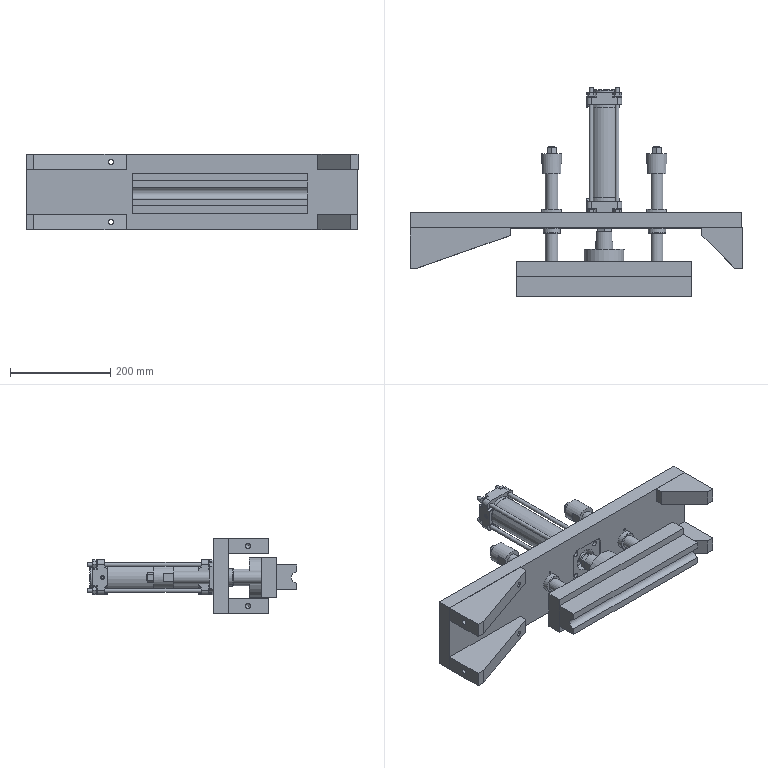Part | NX | features Hexagon Nut ISO - 4034 - M12 - N_Hexagon Nut ISO - 4034 - M12 - N 2, Hydraulic support1 2, Hydraulic support2 2, Hydraulic2.1_50 2, Hydraulic2.2_50 2, Hydraulic2.3_M18X1.5 2, ISO 4762 M16 x 35 --- 35N_ISO 4762 M16 x 35 --- 35N 2, bushing 2, clamp plate 2, clamp shaft 2, clamp stopper 2, plate 2, stifener1 2, stifener2 2, upper clamp 2 | 22 solids | 685 faces | volume 6097092 mm3 | plane 388 | cylinder 214 | cone 76 | spline 5 | torus 2 | commonest cylinder face diameters 4 x34 20 x17 5 x16 6 x16 10.2 x14 8 x12